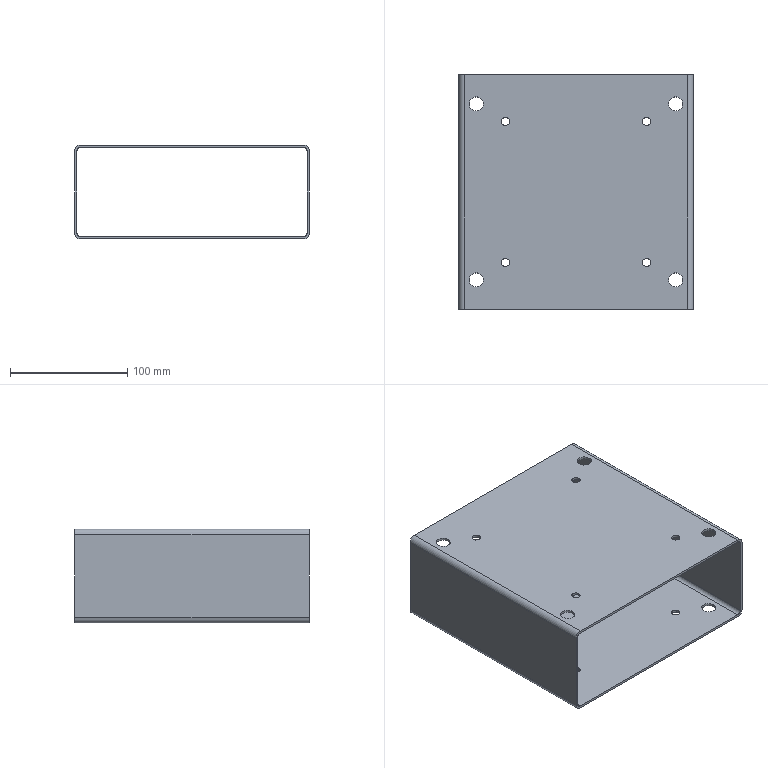Part | STEP file | Fixture seat bracket-PN_0001 | 1 solid | 50 faces | box 200 x 200 x 80 mm | volume 215628 mm3 | cylinder 40 | plane 10 | commonest cylinder face diameters 7 x16 12 x16 6 x4 10 x4